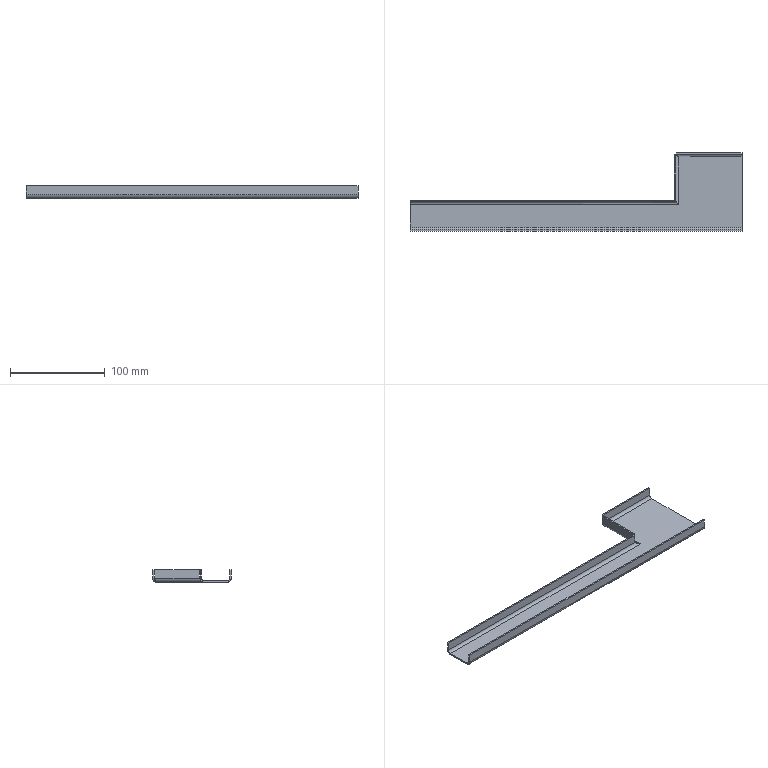Part | SolidWorks | features BaseBody 1 | 1 solid | 40 faces | box 350 x 83 x 13.5 mm | volume 34272 mm3 | plane 28 | cylinder 8 | spline 4 | commonest cylinder face diameters 6 x4 9 x4
STEP:
#1=CARTESIAN_POINT('',(105.707,41.5,12.));
#2=VERTEX_POINT('',#1);
#3=CARTESIAN_POINT('',(105.707,40.,12.));
#4=VERTEX_POINT('',#3);
#5=CARTESIAN_POINT('',(105.707,41.5,12.));
#6=DIRECTION('',(0.,-1.,0.));
#7=VECTOR('',#6,1000.);
#8=LINE('',#5,#7);
#9=EDGE_CURVE('',#2,#4,#8,.T.);
#10=ORIENTED_EDGE('',*,*,#9,.F.);
#11=CARTESIAN_POINT('',(105.707,41.5,3.));
#12=VERTEX_POINT('',#11);
#13=CARTESIAN_POINT('',(105.707,41.5,0.));
#14=DIRECTION('',(0.,0.,1.));
#15=VECTOR('',#14,1000.);
#16=LINE('',#13,#15);
#17=EDGE_CURVE('',#12,#2,#16,.T.);
#18=ORIENTED_EDGE('',*,*,#17,.F.);
#19=CARTESIAN_POINT('',(105.707,40.,3.));
#20=VERTEX_POINT('',#19);
#21=CARTESIAN_POINT('',(105.707,40.,3.));
#22=DIRECTION('',(0.,-1.,0.));
#23=VECTOR('',#22,1000.);
#24=LINE('',#21,#23);
#25=EDGE_CURVE('',#12,#20,#24,.T.);
#26=ORIENTED_EDGE('',*,*,#25,.T.);
#27=CARTESIAN_POINT('',(105.707,40.,0.));
#28=DIRECTION('',(0.,0.,1.));
#29=VECTOR('',#28,1000.);
#30=LINE('',#27,#29);
#31=EDGE_CURVE('',#20,#4,#30,.T.);
#32=ORIENTED_EDGE('',*,*,#31,.T.);
#33=EDGE_LOOP('',(#10,#18,#26,#32));
#34=FACE_OUTER_BOUND('',#33,.T.);
#35=CARTESIAN_POINT('',(105.707,40.,0.));
#36=DIRECTION('',(1.,0.,0.));
#37=DIRECTION('',(0.,1.,0.));
#38=AXIS2_PLACEMENT_3D('',#35,#36,#37);
#39=PLANE('',#38);
#40=ADVANCED_FACE('',(#34),#39,.F.);
#41=CARTESIAN_POINT('',(175.,41.5,12.));
#42=VERTEX_POINT('',#41);
#43=CARTESIAN_POINT('',(175.,41.5,12.));
#44=DIRECTION('',(1.,0.,0.));
#45=VECTOR('',#44,1000.);
#46=LINE('',#43,#45);
#47=EDGE_CURVE('',#2,#42,#46,.T.);
#48=ORIENTED_EDGE('',*,*,#47,.F.);
#49=ORIENTED_EDGE('',*,*,#9,.T.);
#50=CARTESIAN_POINT('',(175.,40.,12.));
#51=VERTEX_POINT('',#50);
#52=CARTESIAN_POINT('',(175.,40.,12.));
#53=DIRECTION('',(1.,0.,0.));
#54=VECTOR('',#53,1000.);
#55=LINE('',#52,#54);
#56=EDGE_CURVE('',#4,#51,#55,.T.);
#57=ORIENTED_EDGE('',*,*,#56,.T.);
#58=CARTESIAN_POINT('',(175.,41.5,12.));
#59=DIRECTION('',(0.,-1.,0.));
#60=VECTOR('',#59,1000.);
#61=LINE('',#58,#60);
#62=EDGE_CURVE('',#42,#51,#61,.T.);
#63=ORIENTED_EDGE('',*,*,#62,.F.);
#64=EDGE_LOOP('',(#48,#49,#57,#63));
#65=FACE_OUTER_BOUND('',#64,.T.);
#66=CARTESIAN_POINT('',(175.,41.5,12.));
#67=DIRECTION('',(0.,0.,-1.));
#68=DIRECTION('',(0.,-1.,0.));
#69=AXIS2_PLACEMENT_3D('',#66,#67,#68);
#70=PLANE('',#69);
#71=ADVANCED_FACE('',(#65),#70,.F.);
#72=ORIENTED_EDGE('',*,*,#31,.F.);
#73=CARTESIAN_POINT('',(175.,40.,3.));
#74=VERTEX_POINT('',#73);
#75=CARTESIAN_POINT('',(175.,40.,3.));
#76=DIRECTION('',(-1.,0.,0.));
#77=VECTOR('',#76,1000.);
#78=LINE('',#75,#77);
#79=EDGE_CURVE('',#74,#20,#78,.T.);
#80=ORIENTED_EDGE('',*,*,#79,.F.);
#81=CARTESIAN_POINT('',(175.,40.,0.));
#82=DIRECTION('',(0.,0.,-1.));
#83=VECTOR('',#82,1000.);
#84=LINE('',#81,#83);
#85=EDGE_CURVE('',#51,#74,#84,.T.);
#86=ORIENTED_EDGE('',*,*,#85,.F.);
#87=ORIENTED_EDGE('',*,*,#56,.F.);
#88=EDGE_LOOP('',(#72,#80,#86,#87));
#89=FACE_OUTER_BOUND('',#88,.T.);
#90=CARTESIAN_POINT('',(0.,40.,0.));
#91=DIRECTION('',(0.,-1.,0.));
#92=DIRECTION('',(-1.,0.,0.));
#93=AXIS2_PLACEMENT_3D('',#90,#91,#92);
#94=PLANE('',#93);
#95=ADVANCED_FACE('',(#89),#94,.T.);
#96=CARTESIAN_POINT('',(175.,41.5,3.));
#97=VERTEX_POINT('',#96);
#98=CARTESIAN_POINT('',(0.,41.5,3.));
#99=DIRECTION('',(1.,0.,0.));
#100=VECTOR('',#99,1000.);
#101=LINE('',#98,#100);
#102=EDGE_CURVE('',#12,#97,#101,.T.);
#103=ORIENTED_EDGE('',*,*,#102,.F.);
#104=ORIENTED_EDGE('',*,*,#17,.T.);
#105=ORIENTED_EDGE('',*,*,#47,.T.);
#106=CARTESIAN_POINT('',(175.,41.5,0.));
#107=DIRECTION('',(0.,0.,-1.));
#108=VECTOR('',#107,1000.);
#109=LINE('',#106,#108);
#110=EDGE_CURVE('',#42,#97,#109,.T.);
#111=ORIENTED_EDGE('',*,*,#110,.T.);
#112=EDGE_LOOP('',(#103,#104,#105,#111));
#113=FACE_OUTER_BOUND('',#112,.T.);
#114=CARTESIAN_POINT('',(0.,41.5,0.));
#115=DIRECTION('',(0.,-1.,0.));
#116=DIRECTION('',(-1.,0.,0.));
#117=AXIS2_PLACEMENT_3D('',#114,#115,#116);
#118=PLANE('',#117);
#119=ADVANCED_FACE('',(#113),#118,.F.);
#120=CARTESIAN_POINT('',(175.,40.,3.));
#121=DIRECTION('',(0.,1.,0.));
#122=VECTOR('',#121,1000.);
#123=LINE('',#120,#122);
#124=EDGE_CURVE('',#74,#97,#123,.T.);
#125=ORIENTED_EDGE('',*,*,#124,.T.);
#126=ORIENTED_EDGE('',*,*,#110,.F.);
#127=ORIENTED_EDGE('',*,*,#62,.T.);
#128=ORIENTED_EDGE('',*,*,#85,.T.);
#129=EDGE_LOOP('',(#125,#126,#127,#128));
#130=FACE_OUTER_BOUND('',#129,.T.);
#131=CARTESIAN_POINT('',(175.,41.5,0.));
#132=DIRECTION('',(-1.,0.,0.));
#133=DIRECTION('',(0.,0.,1.));
#134=AXIS2_PLACEMENT_3D('',#131,#132,#133);
#135=PLANE('',#134);
#136=ADVANCED_FACE('',(#130),#135,.F.);
#137=CARTESIAN_POINT('',(108.,37.,0.));
#138=VERTEX_POINT('',#137);
#139=CARTESIAN_POINT('',(175.,37.,0.));
#140=VERTEX_POINT('',#139);
#141=CARTESIAN_POINT('',(105.707,37.,0.));
#142=DIRECTION('',(1.,0.,0.));
#143=VECTOR('',#142,1000.);
#144=LINE('',#141,#143);
#145=EDGE_CURVE('',#138,#140,#144,.T.);
#146=ORIENTED_EDGE('',*,*,#145,.T.);
#147=CARTESIAN_POINT('',(175.,37.,3.));
#148=DIRECTION('',(1.,0.,0.));
#149=DIRECTION('',(0.,0.,1.));
#150=AXIS2_PLACEMENT_3D('',#147,#148,#149);
#151=CIRCLE('',#150,3.);
#152=EDGE_CURVE('',#140,#74,#151,.T.);
#153=ORIENTED_EDGE('',*,*,#152,.T.);
#154=ORIENTED_EDGE('',*,*,#79,.T.);
#155=CARTESIAN_POINT('',(105.707,40.,3.));
#156=CARTESIAN_POINT('',(105.898,40.,2.607));
#157=CARTESIAN_POINT('',(106.089,39.922,2.215));
#158=CARTESIAN_POINT('',(106.471,39.621,1.489));
#159=CARTESIAN_POINT('',(106.662,39.399,1.156));
#160=CARTESIAN_POINT('',(107.045,38.844,0.601));
#161=CARTESIAN_POINT('',(107.236,38.511,0.3786));
#162=CARTESIAN_POINT('',(107.618,37.785,0.07808));
#163=CARTESIAN_POINT('',(107.809,37.393,0.));
#164=CARTESIAN_POINT('',(108.,37.,0.));
#165=B_SPLINE_CURVE_WITH_KNOTS('',3,(#155,#156,#157,#158,#159,#160,#161,#162,#163,#164),.UNSPECIFIED.,.F.,.F.,(4,2,2,2,4),(0.,0.25,0.5,0.75,1.),.UNSPECIFIED.);
#166=EDGE_CURVE('',#20,#138,#165,.T.);
#167=ORIENTED_EDGE('',*,*,#166,.T.);
#168=EDGE_LOOP('',(#146,#153,#154,#167));
#169=FACE_OUTER_BOUND('',#168,.T.);
#170=CARTESIAN_POINT('',(105.707,37.,3.));
#171=DIRECTION('',(-1.,0.,0.));
#172=DIRECTION('',(0.,1.,0.));
#173=AXIS2_PLACEMENT_3D('',#170,#171,#172);
#174=CYLINDRICAL_SURFACE('',#173,3.);
#175=ADVANCED_FACE('',(#169),#174,.F.);
#176=CARTESIAN_POINT('',(108.,37.,-1.5));
#177=VERTEX_POINT('',#176);
#178=CARTESIAN_POINT('',(175.,37.,-1.5));
#179=VERTEX_POINT('',#178);
#180=CARTESIAN_POINT('',(105.707,37.,-1.5));
#181=DIRECTION('',(1.,0.,0.));
#182=VECTOR('',#181,1000.);
#183=LINE('',#180,#182);
#184=EDGE_CURVE('',#177,#179,#183,.T.);
#185=ORIENTED_EDGE('',*,*,#184,.F.);
#186=CARTESIAN_POINT('',(105.707,41.5,3.));
#187=CARTESIAN_POINT('',(105.898,41.5,2.411));
#188=CARTESIAN_POINT('',(106.089,41.383,1.822));
#189=CARTESIAN_POINT('',(106.471,40.932,0.7337));
#190=CARTESIAN_POINT('',(106.662,40.599,0.2345));
#191=CARTESIAN_POINT('',(107.045,39.765,-0.5985));
#192=CARTESIAN_POINT('',(107.236,39.266,-0.932));
#193=CARTESIAN_POINT('',(107.618,38.178,-1.383));
#194=CARTESIAN_POINT('',(107.809,37.589,-1.5));
#195=CARTESIAN_POINT('',(108.,37.,-1.5));
#196=B_SPLINE_CURVE_WITH_KNOTS('',3,(#186,#187,#188,#189,#190,#191,#192,#193,#194,#195),.UNSPECIFIED.,.F.,.F.,(4,2,2,2,4),(0.,0.25,0.5,0.75,1.),.UNSPECIFIED.);
#197=EDGE_CURVE('',#12,#177,#196,.T.);
#198=ORIENTED_EDGE('',*,*,#197,.F.);
#199=ORIENTED_EDGE('',*,*,#102,.T.);
#200=CARTESIAN_POINT('',(175.,37.,3.));
#201=DIRECTION('',(1.,0.,0.));
#202=DIRECTION('',(0.,0.,1.));
#203=AXIS2_PLACEMENT_3D('',#200,#201,#202);
#204=CIRCLE('',#203,4.5);
#205=EDGE_CURVE('',#179,#97,#204,.T.);
#206=ORIENTED_EDGE('',*,*,#205,.F.);
#207=EDGE_LOOP('',(#185,#198,#199,#206));
#208=FACE_OUTER_BOUND('',#207,.T.);
#209=CARTESIAN_POINT('',(105.707,37.,3.));
#210=DIRECTION('',(-1.,0.,0.));
#211=DIRECTION('',(0.,1.,0.));
#212=AXIS2_PLACEMENT_3D('',#209,#210,#211);
#213=CYLINDRICAL_SURFACE('',#212,4.5);
#214=ADVANCED_FACE('',(#208),#213,.T.);
#215=ORIENTED_EDGE('',*,*,#166,.F.);
#216=ORIENTED_EDGE('',*,*,#25,.F.);
#217=ORIENTED_EDGE('',*,*,#197,.T.);
#218=CARTESIAN_POINT('',(108.,37.,0.));
#219=DIRECTION('',(0.,0.,-1.));
#220=VECTOR('',#219,1000.);
#221=LINE('',#218,#220);
#222=EDGE_CURVE('',#138,#177,#221,.T.);
#223=ORIENTED_EDGE('',*,*,#222,.F.);
#224=EDGE_LOOP('',(#215,#216,#217,#223));
#225=FACE_OUTER_BOUND('',#224,.T.);
#226=CARTESIAN_POINT('',(105.707,41.515,3.));
#227=CARTESIAN_POINT('',(105.898,41.515,2.409));
#228=CARTESIAN_POINT('',(106.089,41.397,1.818));
#229=CARTESIAN_POINT('',(106.471,40.945,0.7262));
#230=CARTESIAN_POINT('',(106.662,40.61,0.2253));
#231=CARTESIAN_POINT('',(107.045,39.775,-0.6105));
#232=CARTESIAN_POINT('',(107.236,39.274,-0.9451));
#233=CARTESIAN_POINT('',(107.618,38.182,-1.397));
#234=CARTESIAN_POINT('',(107.809,37.591,-1.515));
#235=CARTESIAN_POINT('',(108.,37.,-1.515));
#236=CARTESIAN_POINT('',(105.707,41.5,3.));
#237=CARTESIAN_POINT('',(105.898,41.5,2.411));
#238=CARTESIAN_POINT('',(106.089,41.383,1.822));
#239=CARTESIAN_POINT('',(106.471,40.932,0.7337));
#240=CARTESIAN_POINT('',(106.662,40.599,0.2345));
#241=CARTESIAN_POINT('',(107.045,39.765,-0.5985));
#242=CARTESIAN_POINT('',(107.236,39.266,-0.932));
#243=CARTESIAN_POINT('',(107.618,38.178,-1.383));
#244=CARTESIAN_POINT('',(107.809,37.589,-1.5));
#245=CARTESIAN_POINT('',(108.,37.,-1.5));
#246=CARTESIAN_POINT('',(105.707,40.,3.));
#247=CARTESIAN_POINT('',(105.898,40.,2.607));
#248=CARTESIAN_POINT('',(106.089,39.922,2.215));
#249=CARTESIAN_POINT('',(106.471,39.621,1.489));
#250=CARTESIAN_POINT('',(106.662,39.399,1.156));
#251=CARTESIAN_POINT('',(107.045,38.844,0.601));
#252=CARTESIAN_POINT('',(107.236,38.511,0.3786));
#253=CARTESIAN_POINT('',(107.618,37.785,0.07808));
#254=CARTESIAN_POINT('',(107.809,37.393,0.));
#255=CARTESIAN_POINT('',(108.,37.,0.));
#256=CARTESIAN_POINT('',(105.707,39.985,3.));
#257=CARTESIAN_POINT('',(105.898,39.985,2.609));
#258=CARTESIAN_POINT('',(106.089,39.907,2.219));
#259=CARTESIAN_POINT('',(106.471,39.608,1.497));
#260=CARTESIAN_POINT('',(106.662,39.387,1.166));
#261=CARTESIAN_POINT('',(107.045,38.834,0.6131));
#262=CARTESIAN_POINT('',(107.236,38.503,0.3919));
#263=CARTESIAN_POINT('',(107.618,37.781,0.09284));
#264=CARTESIAN_POINT('',(107.809,37.391,0.01515));
#265=CARTESIAN_POINT('',(108.,37.,0.01515));
#266=B_SPLINE_SURFACE_WITH_KNOTS('',1,3,((#226,#227,#228,#229,#230,#231,#232,#233,#234,#235),(#236,#237,#238,#239,#240,#241,#242,#243,#244,#245),(#246,#247,#248,#249,#250,#251,#252,#253,#254,#255),(#256,#257,#258,#259,#260,#261,#262,#263,#264,#265)),.UNSPECIFIED.,.F.,.F.,.F.,(2,1,1,2),(4,2,2,2,4),(-0.01,0.,1.,1.01),(0.,0.25,0.5,0.75,1.),.UNSPECIFIED.);
#267=ADVANCED_FACE('',(#225),#266,.F.);
#268=ORIENTED_EDGE('',*,*,#124,.F.);
#269=ORIENTED_EDGE('',*,*,#152,.F.);
#270=CARTESIAN_POINT('',(175.,37.,0.));
#271=DIRECTION('',(0.,0.,-1.));
#272=VECTOR('',#271,1000.);
#273=LINE('',#270,#272);
#274=EDGE_CURVE('',#140,#179,#273,.T.);
#275=ORIENTED_EDGE('',*,*,#274,.T.);
#276=ORIENTED_EDGE('',*,*,#205,.T.);
#277=EDGE_LOOP('',(#268,#269,#275,#276));
#278=FACE_OUTER_BOUND('',#277,.T.);
#279=CARTESIAN_POINT('',(175.,37.,3.));
#280=DIRECTION('',(1.,0.,0.));
#281=DIRECTION('',(0.,1.,0.));
#282=AXIS2_PLACEMENT_3D('',#279,#280,#281);
#283=PLANE('',#282);
#284=ADVANCED_FACE('',(#278),#283,.T.);
#285=CARTESIAN_POINT('',(103.5,-7.793,12.));
#286=VERTEX_POINT('',#285);
#287=CARTESIAN_POINT('',(105.,-7.793,12.));
#288=VERTEX_POINT('',#287);
#289=CARTESIAN_POINT('',(103.5,-7.793,12.));
#290=DIRECTION('',(1.,0.,0.));
#291=VECTOR('',#290,1000.);
#292=LINE('',#289,#291);
#293=EDGE_CURVE('',#286,#288,#292,.T.);
#294=ORIENTED_EDGE('',*,*,#293,.F.);
#295=CARTESIAN_POINT('',(103.5,-7.793,3.));
#296=VERTEX_POINT('',#295);
#297=CARTESIAN_POINT('',(103.5,-7.793,0.));
#298=DIRECTION('',(0.,0.,1.));
#299=VECTOR('',#298,1000.);
#300=LINE('',#297,#299);
#301=EDGE_CURVE('',#296,#286,#300,.T.);
#302=ORIENTED_EDGE('',*,*,#301,.F.);
#303=CARTESIAN_POINT('',(105.,-7.793,3.));
#304=VERTEX_POINT('',#303);
#305=CARTESIAN_POINT('',(105.,-7.793,3.));
#306=DIRECTION('',(1.,0.,0.));
#307=VECTOR('',#306,1000.);
#308=LINE('',#305,#307);
#309=EDGE_CURVE('',#296,#304,#308,.T.);
#310=ORIENTED_EDGE('',*,*,#309,.T.);
#311=CARTESIAN_POINT('',(105.,-7.793,0.));
#312=DIRECTION('',(0.,0.,1.));
#313=VECTOR('',#312,1000.);
#314=LINE('',#311,#313);
#315=EDGE_CURVE('',#304,#288,#314,.T.);
#316=ORIENTED_EDGE('',*,*,#315,.T.);
#317=EDGE_LOOP('',(#294,#302,#310,#316));
#318=FACE_OUTER_BOUND('',#317,.T.);
#319=CARTESIAN_POINT('',(105.,-7.793,0.));
#320=DIRECTION('',(0.,1.,0.));
#321=DIRECTION('',(1.,0.,0.));
#322=AXIS2_PLACEMENT_3D('',#319,#320,#321);
#323=PLANE('',#322);
#324=ADVANCED_FACE('',(#318),#323,.F.);
#325=CARTESIAN_POINT('',(103.5,39.293,12.));
#326=VERTEX_POINT('',#325);
#327=CARTESIAN_POINT('',(103.5,40.,12.));
#328=DIRECTION('',(0.,1.,0.));
#329=VECTOR('',#328,1000.);
#330=LINE('',#327,#329);
#331=EDGE_CURVE('',#286,#326,#330,.T.);
#332=ORIENTED_EDGE('',*,*,#331,.F.);
#333=ORIENTED_EDGE('',*,*,#293,.T.);
#334=CARTESIAN_POINT('',(105.,39.293,12.));
#335=VERTEX_POINT('',#334);
#336=CARTESIAN_POINT('',(105.,40.,12.));
#337=DIRECTION('',(0.,1.,0.));
#338=VECTOR('',#337,1000.);
#339=LINE('',#336,#338);
#340=EDGE_CURVE('',#288,#335,#339,.T.);
#341=ORIENTED_EDGE('',*,*,#340,.T.);
#342=CARTESIAN_POINT('',(103.5,39.293,12.));
#343=DIRECTION('',(1.,0.,0.));
#344=VECTOR('',#343,1000.);
#345=LINE('',#342,#344);
#346=EDGE_CURVE('',#326,#335,#345,.T.);
#347=ORIENTED_EDGE('',*,*,#346,.F.);
#348=EDGE_LOOP('',(#332,#333,#341,#347));
#349=FACE_OUTER_BOUND('',#348,.T.);
#350=CARTESIAN_POINT('',(103.5,40.,12.));
#351=DIRECTION('',(0.,0.,-1.));
#352=DIRECTION('',(0.,-1.,0.));
#353=AXIS2_PLACEMENT_3D('',#350,#351,#352);
#354=PLANE('',#353);
#355=ADVANCED_FACE('',(#349),#354,.F.);
#356=ORIENTED_EDGE('',*,*,#315,.F.);
#357=CARTESIAN_POINT('',(105.,39.293,3.));
#358=VERTEX_POINT('',#357);
#359=CARTESIAN_POINT('',(105.,40.,3.));
#360=DIRECTION('',(0.,-1.,0.));
#361=VECTOR('',#360,1000.);
#362=LINE('',#359,#361);
#363=EDGE_CURVE('',#358,#304,#362,.T.);
#364=ORIENTED_EDGE('',*,*,#363,.F.);
#365=CARTESIAN_POINT('',(105.,39.293,0.));
#366=DIRECTION('',(0.,0.,1.));
#367=VECTOR('',#366,1000.);
#368=LINE('',#365,#367);
#369=EDGE_CURVE('',#358,#335,#368,.T.);
#370=ORIENTED_EDGE('',*,*,#369,.T.);
#371=ORIENTED_EDGE('',*,*,#340,.F.);
#372=EDGE_LOOP('',(#356,#364,#370,#371));
#373=FACE_OUTER_BOUND('',#372,.T.);
#374=CARTESIAN_POINT('',(105.,0.,0.));
#375=DIRECTION('',(1.,0.,0.));
#376=DIRECTION('',(0.,0.,1.));
#377=AXIS2_PLACEMENT_3D('',#374,#375,#376);
#378=PLANE('',#377);
#379=ADVANCED_FACE('',(#373),#378,.T.);
#380=CARTESIAN_POINT('',(103.5,39.293,3.));
#381=VERTEX_POINT('',#380);
#382=CARTESIAN_POINT('',(103.5,0.,3.));
#383=DIRECTION('',(0.,1.,0.));
#384=VECTOR('',#383,1000.);
#385=LINE('',#382,#384);
#386=EDGE_CURVE('',#296,#381,#385,.T.);
#387=ORIENTED_EDGE('',*,*,#386,.F.);
#388=ORIENTED_EDGE('',*,*,#301,.T.);
#389=ORIENTED_EDGE('',*,*,#331,.T.);
#390=CARTESIAN_POINT('',(103.5,39.293,0.));
#391=DIRECTION('',(0.,0.,1.));
#392=VECTOR('',#391,1000.);
#393=LINE('',#390,#392);
#394=EDGE_CURVE('',#381,#326,#393,.T.);
#395=ORIENTED_EDGE('',*,*,#394,.F.);
#396=EDGE_LOOP('',(#387,#388,#389,#395));
#397=FACE_OUTER_BOUND('',#396,.T.);
#398=CARTESIAN_POINT('',(103.5,0.,0.));
#399=DIRECTION('',(1.,0.,0.));
#400=DIRECTION('',(0.,0.,1.));
#401=AXIS2_PLACEMENT_3D('',#398,#399,#400);
#402=PLANE('',#401);
#403=ADVANCED_FACE('',(#397),#402,.F.);
#404=ORIENTED_EDGE('',*,*,#394,.T.);
#405=ORIENTED_EDGE('',*,*,#346,.T.);
#406=ORIENTED_EDGE('',*,*,#369,.F.);
#407=CARTESIAN_POINT('',(105.,39.293,3.));
#408=DIRECTION('',(1.,0.,0.));
#409=VECTOR('',#408,1000.);
#410=LINE('',#407,#409);
#411=EDGE_CURVE('',#381,#358,#410,.T.);
#412=ORIENTED_EDGE('',*,*,#411,.F.);
#413=EDGE_LOOP('',(#404,#405,#406,#412));
#414=FACE_OUTER_BOUND('',#413,.T.);
#415=CARTESIAN_POINT('',(105.,39.293,0.));
#416=DIRECTION('',(0.,1.,0.));
#417=DIRECTION('',(1.,0.,0.));
#418=AXIS2_PLACEMENT_3D('',#415,#416,#417);
#419=PLANE('',#418);
#420=ADVANCED_FACE('',(#414),#419,.T.);
#421=CARTESIAN_POINT('',(108.,-13.,0.));
#422=VERTEX_POINT('',#421);
#423=CARTESIAN_POINT('',(108.,-13.,0.));
#424=DIRECTION('',(0.,1.,0.));
#425=VECTOR('',#424,1000.);
#426=LINE('',#423,#425);
#427=EDGE_CURVE('',#422,#138,#426,.T.);
#428=ORIENTED_EDGE('',*,*,#427,.T.);
#429=CARTESIAN_POINT('',(108.,37.,0.));
#430=CARTESIAN_POINT('',(107.607,37.191,0.));
#431=CARTESIAN_POINT('',(107.215,37.382,0.07808));
#432=CARTESIAN_POINT('',(106.489,37.764,0.3786));
#433=CARTESIAN_POINT('',(106.156,37.955,0.601));
#434=CARTESIAN_POINT('',(105.601,38.338,1.156));
#435=CARTESIAN_POINT('',(105.379,38.529,1.489));
#436=CARTESIAN_POINT('',(105.078,38.911,2.215));
#437=CARTESIAN_POINT('',(105.,39.102,2.607));
#438=CARTESIAN_POINT('',(105.,39.293,3.));
#439=B_SPLINE_CURVE_WITH_KNOTS('',3,(#429,#430,#431,#432,#433,#434,#435,#436,#437,#438),.UNSPECIFIED.,.F.,.F.,(4,2,2,2,4),(0.,0.25,0.5,0.75,1.),.UNSPECIFIED.);
#440=EDGE_CURVE('',#138,#358,#439,.T.);
#441=ORIENTED_EDGE('',*,*,#440,.T.);
#442=ORIENTED_EDGE('',*,*,#363,.T.);
#443=CARTESIAN_POINT('',(105.,-7.793,3.));
#444=CARTESIAN_POINT('',(105.,-8.227,2.607));
#445=CARTESIAN_POINT('',(105.078,-8.661,2.215));
#446=CARTESIAN_POINT('',(105.379,-9.529,1.489));
#447=CARTESIAN_POINT('',(105.601,-9.963,1.156));
#448=CARTESIAN_POINT('',(106.156,-10.83,0.601));
#449=CARTESIAN_POINT('',(106.489,-11.264,0.3786));
#450=CARTESIAN_POINT('',(107.215,-12.132,0.07808));
#451=CARTESIAN_POINT('',(107.607,-12.566,0.));
#452=CARTESIAN_POINT('',(108.,-13.,0.));
#453=B_SPLINE_CURVE_WITH_KNOTS('',3,(#443,#444,#445,#446,#447,#448,#449,#450,#451,#452),.UNSPECIFIED.,.F.,.F.,(4,2,2,2,4),(0.,0.25,0.5,0.75,1.),.UNSPECIFIED.);
#454=EDGE_CURVE('',#304,#422,#453,.T.);
#455=ORIENTED_EDGE('',*,*,#454,.T.);
#456=EDGE_LOOP('',(#428,#441,#442,#455));
#457=FACE_OUTER_BOUND('',#456,.T.);
#458=CARTESIAN_POINT('',(108.,-13.,3.));
#459=DIRECTION('',(0.,-1.,0.));
#460=DIRECTION('',(-1.,0.,0.));
#461=AXIS2_PLACEMENT_3D('',#458,#459,#460);
#462=CYLINDRICAL_SURFACE('',#461,3.);
#463=ADVANCED_FACE('',(#457),#462,.F.);
#464=CARTESIAN_POINT('',(108.,-13.,-1.5));
#465=VERTEX_POINT('',#464);
#466=CARTESIAN_POINT('',(108.,-13.,-1.5));
#467=DIRECTION('',(0.,1.,0.));
#468=VECTOR('',#467,1000.);
#469=LINE('',#466,#468);
#470=EDGE_CURVE('',#465,#177,#469,.T.);
#471=ORIENTED_EDGE('',*,*,#470,.F.);
#472=CARTESIAN_POINT('',(103.5,-7.793,3.));
#473=CARTESIAN_POINT('',(103.5,-8.227,2.411));
#474=CARTESIAN_POINT('',(103.617,-8.661,1.822));
#475=CARTESIAN_POINT('',(104.068,-9.529,0.7337));
#476=CARTESIAN_POINT('',(104.401,-9.963,0.2345));
#477=CARTESIAN_POINT('',(105.235,-10.83,-0.5985));
#478=CARTESIAN_POINT('',(105.734,-11.264,-0.932));
#479=CARTESIAN_POINT('',(106.822,-12.132,-1.383));
#480=CARTESIAN_POINT('',(107.411,-12.566,-1.5));
#481=CARTESIAN_POINT('',(108.,-13.,-1.5));
#482=B_SPLINE_CURVE_WITH_KNOTS('',3,(#472,#473,#474,#475,#476,#477,#478,#479,#480,#481),.UNSPECIFIED.,.F.,.F.,(4,2,2,2,4),(0.,0.25,0.5,0.75,1.),.UNSPECIFIED.);
#483=EDGE_CURVE('',#296,#465,#482,.T.);
#484=ORIENTED_EDGE('',*,*,#483,.F.);
#485=ORIENTED_EDGE('',*,*,#386,.T.);
#486=CARTESIAN_POINT('',(108.,37.,-1.5));
#487=CARTESIAN_POINT('',(107.411,37.191,-1.5));
#488=CARTESIAN_POINT('',(106.822,37.382,-1.383));
#489=CARTESIAN_POINT('',(105.734,37.764,-0.932));
#490=CARTESIAN_POINT('',(105.235,37.955,-0.5985));
#491=CARTESIAN_POINT('',(104.401,38.338,0.2345));
#492=CARTESIAN_POINT('',(104.068,38.529,0.7337));
#493=CARTESIAN_POINT('',(103.617,38.911,1.822));
#494=CARTESIAN_POINT('',(103.5,39.102,2.411));
#495=CARTESIAN_POINT('',(103.5,39.293,3.));
#496=B_SPLINE_CURVE_WITH_KNOTS('',3,(#486,#487,#488,#489,#490,#491,#492,#493,#494,#495),.UNSPECIFIED.,.F.,.F.,(4,2,2,2,4),(0.,0.25,0.5,0.75,1.),.UNSPECIFIED.);
#497=EDGE_CURVE('',#177,#381,#496,.T.);
#498=ORIENTED_EDGE('',*,*,#497,.F.);
#499=EDGE_LOOP('',(#471,#484,#485,#498));
#500=FACE_OUTER_BOUND('',#499,.T.);
#501=CARTESIAN_POINT('',(108.,-13.,3.));
#502=DIRECTION('',(0.,-1.,0.));
#503=DIRECTION('',(-1.,0.,0.));
#504=AXIS2_PLACEMENT_3D('',#501,#502,#503);
#505=CYLINDRICAL_SURFACE('',#504,4.5);
#506=ADVANCED_FACE('',(#500),#505,.T.);
#507=ORIENTED_EDGE('',*,*,#454,.F.);
#508=ORIENTED_EDGE('',*,*,#309,.F.);
#509=ORIENTED_EDGE('',*,*,#483,.T.);
#510=CARTESIAN_POINT('',(108.,-13.,0.));
#511=DIRECTION('',(0.,0.,-1.));
#512=VECTOR('',#511,1000.);
#513=LINE('',#510,#512);
#514=EDGE_CURVE('',#422,#465,#513,.T.);
#515=ORIENTED_EDGE('',*,*,#514,.F.);
#516=EDGE_LOOP('',(#507,#508,#509,#515));
#517=FACE_OUTER_BOUND('',#516,.T.);
#518=CARTESIAN_POINT('',(103.485,-7.793,3.));
#519=CARTESIAN_POINT('',(103.485,-8.227,2.409));
#520=CARTESIAN_POINT('',(103.603,-8.661,1.818));
#521=CARTESIAN_POINT('',(104.055,-9.529,0.7262));
#522=CARTESIAN_POINT('',(104.39,-9.963,0.2253));
#523=CARTESIAN_POINT('',(105.225,-10.83,-0.6105));
#524=CARTESIAN_POINT('',(105.726,-11.264,-0.9451));
#525=CARTESIAN_POINT('',(106.818,-12.132,-1.397));
#526=CARTESIAN_POINT('',(107.409,-12.566,-1.515));
#527=CARTESIAN_POINT('',(108.,-13.,-1.515));
#528=CARTESIAN_POINT('',(103.5,-7.793,3.));
#529=CARTESIAN_POINT('',(103.5,-8.227,2.411));
#530=CARTESIAN_POINT('',(103.617,-8.661,1.822));
#531=CARTESIAN_POINT('',(104.068,-9.529,0.7337));
#532=CARTESIAN_POINT('',(104.401,-9.963,0.2345));
#533=CARTESIAN_POINT('',(105.235,-10.83,-0.5985));
#534=CARTESIAN_POINT('',(105.734,-11.264,-0.932));
#535=CARTESIAN_POINT('',(106.822,-12.132,-1.383));
#536=CARTESIAN_POINT('',(107.411,-12.566,-1.5));
#537=CARTESIAN_POINT('',(108.,-13.,-1.5));
#538=CARTESIAN_POINT('',(105.,-7.793,3.));
#539=CARTESIAN_POINT('',(105.,-8.227,2.607));
#540=CARTESIAN_POINT('',(105.078,-8.661,2.215));
#541=CARTESIAN_POINT('',(105.379,-9.529,1.489));
#542=CARTESIAN_POINT('',(105.601,-9.963,1.156));
#543=CARTESIAN_POINT('',(106.156,-10.83,0.601));
#544=CARTESIAN_POINT('',(106.489,-11.264,0.3786));
#545=CARTESIAN_POINT('',(107.215,-12.132,0.07808));
#546=CARTESIAN_POINT('',(107.607,-12.566,0.));
#547=CARTESIAN_POINT('',(108.,-13.,0.));
#548=CARTESIAN_POINT('',(105.015,-7.793,3.));
#549=CARTESIAN_POINT('',(105.015,-8.227,2.609));
#550=CARTESIAN_POINT('',(105.093,-8.661,2.219));
#551=CARTESIAN_POINT('',(105.392,-9.529,1.497));
#552=CARTESIAN_POINT('',(105.613,-9.963,1.166));
#553=CARTESIAN_POINT('',(106.166,-10.83,0.6131));
#554=CARTESIAN_POINT('',(106.497,-11.264,0.3919));
#555=CARTESIAN_POINT('',(107.219,-12.132,0.09284));
#556=CARTESIAN_POINT('',(107.609,-12.566,0.01515));
#557=CARTESIAN_POINT('',(108.,-13.,0.01515));
#558=B_SPLINE_SURFACE_WITH_KNOTS('',1,3,((#518,#519,#520,#521,#522,#523,#524,#525,#526,#527),(#528,#529,#530,#531,#532,#533,#534,#535,#536,#537),(#538,#539,#540,#541,#542,#543,#544,#545,#546,#547),(#548,#549,#550,#551,#552,#553,#554,#555,#556,#557)),.UNSPECIFIED.,.F.,.F.,.F.,(2,1,1,2),(4,2,2,2,4),(-0.01,0.,1.,1.01),(0.,0.25,0.5,0.75,1.),.UNSPECIFIED.);
#559=ADVANCED_FACE('',(#517),#558,.F.);
#560=ORIENTED_EDGE('',*,*,#411,.T.);
#561=ORIENTED_EDGE('',*,*,#440,.F.);
#562=ORIENTED_EDGE('',*,*,#222,.T.);
#563=ORIENTED_EDGE('',*,*,#497,.T.);
#564=EDGE_LOOP('',(#560,#561,#562,#563));
#565=FACE_OUTER_BOUND('',#564,.T.);
#566=CARTESIAN_POINT('',(108.,37.,-1.515));
#567=CARTESIAN_POINT('',(107.409,37.191,-1.515));
#568=CARTESIAN_POINT('',(106.818,37.382,-1.397));
#569=CARTESIAN_POINT('',(105.726,37.764,-0.9451));
#570=CARTESIAN_POINT('',(105.225,37.955,-0.6105));
#571=CARTESIAN_POINT('',(104.39,38.338,0.2253));
#572=CARTESIAN_POINT('',(104.055,38.529,0.7262));
#573=CARTESIAN_POINT('',(103.603,38.911,1.818));
#574=CARTESIAN_POINT('',(103.485,39.102,2.409));
#575=CARTESIAN_POINT('',(103.485,39.293,3.));
#576=CARTESIAN_POINT('',(108.,37.,-1.5));
#577=CARTESIAN_POINT('',(107.411,37.191,-1.5));
#578=CARTESIAN_POINT('',(106.822,37.382,-1.383));
#579=CARTESIAN_POINT('',(105.734,37.764,-0.932));
#580=CARTESIAN_POINT('',(105.235,37.955,-0.5985));
#581=CARTESIAN_POINT('',(104.401,38.338,0.2345));
#582=CARTESIAN_POINT('',(104.068,38.529,0.7337));
#583=CARTESIAN_POINT('',(103.617,38.911,1.822));
#584=CARTESIAN_POINT('',(103.5,39.102,2.411));
#585=CARTESIAN_POINT('',(103.5,39.293,3.));
#586=CARTESIAN_POINT('',(108.,37.,0.));
#587=CARTESIAN_POINT('',(107.607,37.191,0.));
#588=CARTESIAN_POINT('',(107.215,37.382,0.07808));
#589=CARTESIAN_POINT('',(106.489,37.764,0.3786));
#590=CARTESIAN_POINT('',(106.156,37.955,0.601));
#591=CARTESIAN_POINT('',(105.601,38.338,1.156));
#592=CARTESIAN_POINT('',(105.379,38.529,1.489));
#593=CARTESIAN_POINT('',(105.078,38.911,2.215));
#594=CARTESIAN_POINT('',(105.,39.102,2.607));
#595=CARTESIAN_POINT('',(105.,39.293,3.));
#596=CARTESIAN_POINT('',(108.,37.,0.01515));
#597=CARTESIAN_POINT('',(107.609,37.191,0.01515));
#598=CARTESIAN_POINT('',(107.219,37.382,0.09284));
#599=CARTESIAN_POINT('',(106.497,37.764,0.3919));
#600=CARTESIAN_POINT('',(106.166,37.955,0.6131));
#601=CARTESIAN_POINT('',(105.613,38.338,1.166));
#602=CARTESIAN_POINT('',(105.392,38.529,1.497));
#603=CARTESIAN_POINT('',(105.093,38.911,2.219));
#604=CARTESIAN_POINT('',(105.015,39.102,2.609));
#605=CARTESIAN_POINT('',(105.015,39.293,3.));
#606=B_SPLINE_SURFACE_WITH_KNOTS('',1,3,((#566,#567,#568,#569,#570,#571,#572,#573,#574,#575),(#576,#577,#578,#579,#580,#581,#582,#583,#584,#585),(#586,#587,#588,#589,#590,#591,#592,#593,#594,#595),(#596,#597,#598,#599,#600,#601,#602,#603,#604,#605)),.UNSPECIFIED.,.F.,.F.,.F.,(2,1,1,2),(4,2,2,2,4),(-0.01,0.,1.,1.01),(0.,0.25,0.5,0.75,1.),.UNSPECIFIED.);
#607=ADVANCED_FACE('',(#565),#606,.F.);
#608=CARTESIAN_POINT('',(-175.,-10.,3.));
#609=VERTEX_POINT('',#608);
#610=CARTESIAN_POINT('',(-175.,-8.5,3.));
#611=VERTEX_POINT('',#610);
#612=CARTESIAN_POINT('',(-175.,-10.,3.));
#613=DIRECTION('',(0.,1.,0.));
#614=VECTOR('',#613,1000.);
#615=LINE('',#612,#614);
#616=EDGE_CURVE('',#609,#611,#615,.T.);
#617=ORIENTED_EDGE('',*,*,#616,.F.);
#618=CARTESIAN_POINT('',(-175.,-10.,12.));
#619=VERTEX_POINT('',#618);
#620=CARTESIAN_POINT('',(-175.,-10.,12.));
#621=DIRECTION('',(0.,0.,1.));
#622=VECTOR('',#621,1000.);
#623=LINE('',#620,#622);
#624=EDGE_CURVE('',#609,#619,#623,.T.);
#625=ORIENTED_EDGE('',*,*,#624,.T.);
#626=CARTESIAN_POINT('',(-175.,-8.5,12.));
#627=VERTEX_POINT('',#626);
#628=CARTESIAN_POINT('',(-175.,-8.5,12.));
#629=DIRECTION('',(0.,-1.,0.));
#630=VECTOR('',#629,1000.);
#631=LINE('',#628,#630);
#632=EDGE_CURVE('',#627,#619,#631,.T.);
#633=ORIENTED_EDGE('',*,*,#632,.F.);
#634=CARTESIAN_POINT('',(-175.,-8.5,12.));
#635=DIRECTION('',(0.,0.,1.));
#636=VECTOR('',#635,1000.);
#637=LINE('',#634,#636);
#638=EDGE_CURVE('',#611,#627,#637,.T.);
#639=ORIENTED_EDGE('',*,*,#638,.F.);
#640=EDGE_LOOP('',(#617,#625,#633,#639));
#641=FACE_OUTER_BOUND('',#640,.T.);
#642=CARTESIAN_POINT('',(-175.,-8.5,12.));
#643=DIRECTION('',(1.,0.,0.));
#644=DIRECTION('',(0.,1.,0.));
#645=AXIS2_PLACEMENT_3D('',#642,#643,#644);
#646=PLANE('',#645);
#647=ADVANCED_FACE('',(#641),#646,.F.);
#648=CARTESIAN_POINT('',(102.793,-8.5,12.));
#649=VERTEX_POINT('',#648);
#650=CARTESIAN_POINT('',(102.793,-10.,12.));
#651=VERTEX_POINT('',#650);
#652=CARTESIAN_POINT('',(102.793,-8.5,12.));
#653=DIRECTION('',(0.,-1.,0.));
#654=VECTOR('',#653,1000.);
#655=LINE('',#652,#654);
#656=EDGE_CURVE('',#649,#651,#655,.T.);
#657=ORIENTED_EDGE('',*,*,#656,.F.);
#658=CARTESIAN_POINT('',(105.,-8.5,12.));
#659=DIRECTION('',(1.,0.,0.));
#660=VECTOR('',#659,1000.);
#661=LINE('',#658,#660);
#662=EDGE_CURVE('',#627,#649,#661,.T.);
#663=ORIENTED_EDGE('',*,*,#662,.F.);
#664=ORIENTED_EDGE('',*,*,#632,.T.);
#665=CARTESIAN_POINT('',(105.,-10.,12.));
#666=DIRECTION('',(1.,0.,0.));
#667=VECTOR('',#666,1000.);
#668=LINE('',#665,#667);
#669=EDGE_CURVE('',#619,#651,#668,.T.);
#670=ORIENTED_EDGE('',*,*,#669,.T.);
#671=EDGE_LOOP('',(#657,#663,#664,#670));
#672=FACE_OUTER_BOUND('',#671,.T.);
#673=CARTESIAN_POINT('',(105.,-8.5,12.));
#674=DIRECTION('',(0.,0.,-1.));
#675=DIRECTION('',(0.,-1.,0.));
#676=AXIS2_PLACEMENT_3D('',#673,#674,#675);
#677=PLANE('',#676);
#678=ADVANCED_FACE('',(#672),#677,.F.);
#679=CARTESIAN_POINT('',(102.793,-10.,3.));
#680=VERTEX_POINT('',#679);
#681=CARTESIAN_POINT('',(105.,-10.,3.));
#682=DIRECTION('',(-1.,0.,0.));
#683=VECTOR('',#682,1000.);
#684=LINE('',#681,#683);
#685=EDGE_CURVE('',#680,#609,#684,.T.);
#686=ORIENTED_EDGE('',*,*,#685,.F.);
#687=CARTESIAN_POINT('',(102.793,-10.,0.));
#688=DIRECTION('',(0.,0.,1.));
#689=VECTOR('',#688,1000.);
#690=LINE('',#687,#689);
#691=EDGE_CURVE('',#680,#651,#690,.T.);
#692=ORIENTED_EDGE('',*,*,#691,.T.);
#693=ORIENTED_EDGE('',*,*,#669,.F.);
#694=ORIENTED_EDGE('',*,*,#624,.F.);
#695=EDGE_LOOP('',(#686,#692,#693,#694));
#696=FACE_OUTER_BOUND('',#695,.T.);
#697=CARTESIAN_POINT('',(0.,-10.,0.));
#698=DIRECTION('',(0.,-1.,0.));
#699=DIRECTION('',(-1.,0.,0.));
#700=AXIS2_PLACEMENT_3D('',#697,#698,#699);
#701=PLANE('',#700);
#702=ADVANCED_FACE('',(#696),#701,.T.);
#703=CARTESIAN_POINT('',(102.793,-8.5,3.));
#704=VERTEX_POINT('',#703);
#705=CARTESIAN_POINT('',(102.793,-8.5,0.));
#706=DIRECTION('',(0.,0.,1.));
#707=VECTOR('',#706,1000.);
#708=LINE('',#705,#707);
#709=EDGE_CURVE('',#704,#649,#708,.T.);
#710=ORIENTED_EDGE('',*,*,#709,.F.);
#711=CARTESIAN_POINT('',(0.,-8.5,3.));
#712=DIRECTION('',(1.,0.,0.));
#713=VECTOR('',#712,1000.);
#714=LINE('',#711,#713);
#715=EDGE_CURVE('',#611,#704,#714,.T.);
#716=ORIENTED_EDGE('',*,*,#715,.F.);
#717=ORIENTED_EDGE('',*,*,#638,.T.);
#718=ORIENTED_EDGE('',*,*,#662,.T.);
#719=EDGE_LOOP('',(#710,#716,#717,#718));
#720=FACE_OUTER_BOUND('',#719,.T.);
#721=CARTESIAN_POINT('',(0.,-8.5,0.));
#722=DIRECTION('',(0.,-1.,0.));
#723=DIRECTION('',(-1.,0.,0.));
#724=AXIS2_PLACEMENT_3D('',#721,#722,#723);
#725=PLANE('',#724);
#726=ADVANCED_FACE('',(#720),#725,.F.);
#727=ORIENTED_EDGE('',*,*,#709,.T.);
#728=ORIENTED_EDGE('',*,*,#656,.T.);
#729=ORIENTED_EDGE('',*,*,#691,.F.);
#730=CARTESIAN_POINT('',(102.793,-10.,3.));
#731=DIRECTION('',(0.,-1.,0.));
#732=VECTOR('',#731,1000.);
#733=LINE('',#730,#732);
#734=EDGE_CURVE('',#704,#680,#733,.T.);
#735=ORIENTED_EDGE('',*,*,#734,.F.);
#736=EDGE_LOOP('',(#727,#728,#729,#735));
#737=FACE_OUTER_BOUND('',#736,.T.);
#738=CARTESIAN_POINT('',(102.793,-10.,0.));
#739=DIRECTION('',(1.,0.,0.));
#740=DIRECTION('',(0.,1.,0.));
#741=AXIS2_PLACEMENT_3D('',#738,#739,#740);
#742=PLANE('',#741);
#743=ADVANCED_FACE('',(#737),#742,.T.);
#744=CARTESIAN_POINT('',(-175.,-13.,0.));
#745=VERTEX_POINT('',#744);
#746=CARTESIAN_POINT('',(-175.,-13.,0.));
#747=DIRECTION('',(1.,0.,0.));
#748=VECTOR('',#747,1000.);
#749=LINE('',#746,#748);
#750=EDGE_CURVE('',#745,#422,#749,.T.);
#751=ORIENTED_EDGE('',*,*,#750,.T.);
#752=CARTESIAN_POINT('',(108.,-13.,0.));
#753=CARTESIAN_POINT('',(107.566,-12.607,0.));
#754=CARTESIAN_POINT('',(107.132,-12.215,0.07808));
#755=CARTESIAN_POINT('',(106.264,-11.489,0.3786));
#756=CARTESIAN_POINT('',(105.83,-11.156,0.601));
#757=CARTESIAN_POINT('',(104.963,-10.601,1.156));
#758=CARTESIAN_POINT('',(104.529,-10.379,1.489));
#759=CARTESIAN_POINT('',(103.661,-10.078,2.215));
#760=CARTESIAN_POINT('',(103.227,-10.,2.607));
#761=CARTESIAN_POINT('',(102.793,-10.,3.));
#762=B_SPLINE_CURVE_WITH_KNOTS('',3,(#752,#753,#754,#755,#756,#757,#758,#759,#760,#761),.UNSPECIFIED.,.F.,.F.,(4,2,2,2,4),(0.,0.25,0.5,0.75,1.),.UNSPECIFIED.);
#763=EDGE_CURVE('',#422,#680,#762,.T.);
#764=ORIENTED_EDGE('',*,*,#763,.T.);
#765=ORIENTED_EDGE('',*,*,#685,.T.);
#766=CARTESIAN_POINT('',(-175.,-13.,3.));
#767=DIRECTION('',(-1.,0.,0.));
#768=DIRECTION('',(0.,0.,1.));
#769=AXIS2_PLACEMENT_3D('',#766,#767,#768);
#770=CIRCLE('',#769,3.);
#771=EDGE_CURVE('',#609,#745,#770,.T.);
#772=ORIENTED_EDGE('',*,*,#771,.T.);
#773=EDGE_LOOP('',(#751,#764,#765,#772));
#774=FACE_OUTER_BOUND('',#773,.T.);
#775=CARTESIAN_POINT('',(-175.,-13.,3.));
#776=DIRECTION('',(-1.,0.,0.));
#777=DIRECTION('',(0.,1.,0.));
#778=AXIS2_PLACEMENT_3D('',#775,#776,#777);
#779=CYLINDRICAL_SURFACE('',#778,3.);
#780=ADVANCED_FACE('',(#774),#779,.F.);
#781=CARTESIAN_POINT('',(-175.,-13.,-1.5));
#782=VERTEX_POINT('',#781);
#783=CARTESIAN_POINT('',(-175.,-13.,-1.5));
#784=DIRECTION('',(1.,0.,0.));
#785=VECTOR('',#784,1000.);
#786=LINE('',#783,#785);
#787=EDGE_CURVE('',#782,#465,#786,.T.);
#788=ORIENTED_EDGE('',*,*,#787,.F.);
#789=CARTESIAN_POINT('',(-175.,-13.,3.));
#790=DIRECTION('',(-1.,0.,0.));
#791=DIRECTION('',(0.,0.,1.));
#792=AXIS2_PLACEMENT_3D('',#789,#790,#791);
#793=CIRCLE('',#792,4.5);
#794=EDGE_CURVE('',#611,#782,#793,.T.);
#795=ORIENTED_EDGE('',*,*,#794,.F.);
#796=ORIENTED_EDGE('',*,*,#715,.T.);
#797=CARTESIAN_POINT('',(108.,-13.,-1.5));
#798=CARTESIAN_POINT('',(107.566,-12.411,-1.5));
#799=CARTESIAN_POINT('',(107.132,-11.822,-1.383));
#800=CARTESIAN_POINT('',(106.264,-10.734,-0.932));
#801=CARTESIAN_POINT('',(105.83,-10.235,-0.5985));
#802=CARTESIAN_POINT('',(104.963,-9.401,0.2345));
#803=CARTESIAN_POINT('',(104.529,-9.068,0.7337));
#804=CARTESIAN_POINT('',(103.661,-8.617,1.822));
#805=CARTESIAN_POINT('',(103.227,-8.5,2.411));
#806=CARTESIAN_POINT('',(102.793,-8.5,3.));
#807=B_SPLINE_CURVE_WITH_KNOTS('',3,(#797,#798,#799,#800,#801,#802,#803,#804,#805,#806),.UNSPECIFIED.,.F.,.F.,(4,2,2,2,4),(0.,0.25,0.5,0.75,1.),.UNSPECIFIED.);
#808=EDGE_CURVE('',#465,#704,#807,.T.);
#809=ORIENTED_EDGE('',*,*,#808,.F.);
#810=EDGE_LOOP('',(#788,#795,#796,#809));
#811=FACE_OUTER_BOUND('',#810,.T.);
#812=CARTESIAN_POINT('',(-175.,-13.,3.));
#813=DIRECTION('',(-1.,0.,0.));
#814=DIRECTION('',(0.,1.,0.));
#815=AXIS2_PLACEMENT_3D('',#812,#813,#814);
#816=CYLINDRICAL_SURFACE('',#815,4.5);
#817=ADVANCED_FACE('',(#811),#816,.T.);
#818=ORIENTED_EDGE('',*,*,#771,.F.);
#819=ORIENTED_EDGE('',*,*,#616,.T.);
#820=ORIENTED_EDGE('',*,*,#794,.T.);
#821=CARTESIAN_POINT('',(-175.,-13.,0.));
#822=DIRECTION('',(0.,0.,-1.));
#823=VECTOR('',#822,1000.);
#824=LINE('',#821,#823);
#825=EDGE_CURVE('',#745,#782,#824,.T.);
#826=ORIENTED_EDGE('',*,*,#825,.F.);
#827=EDGE_LOOP('',(#818,#819,#820,#826));
#828=FACE_OUTER_BOUND('',#827,.T.);
#829=CARTESIAN_POINT('',(-175.,-13.,3.));
#830=DIRECTION('',(1.,0.,0.));
#831=DIRECTION('',(0.,1.,0.));
#832=AXIS2_PLACEMENT_3D('',#829,#830,#831);
#833=PLANE('',#832);
#834=ADVANCED_FACE('',(#828),#833,.F.);
#835=ORIENTED_EDGE('',*,*,#734,.T.);
#836=ORIENTED_EDGE('',*,*,#763,.F.);
#837=ORIENTED_EDGE('',*,*,#514,.T.);
#838=ORIENTED_EDGE('',*,*,#808,.T.);
#839=EDGE_LOOP('',(#835,#836,#837,#838));
#840=FACE_OUTER_BOUND('',#839,.T.);
#841=CARTESIAN_POINT('',(108.,-13.,-1.515));
#842=CARTESIAN_POINT('',(107.566,-12.409,-1.515));
#843=CARTESIAN_POINT('',(107.132,-11.818,-1.397));
#844=CARTESIAN_POINT('',(106.264,-10.726,-0.9451));
#845=CARTESIAN_POINT('',(105.83,-10.225,-0.6105));
#846=CARTESIAN_POINT('',(104.963,-9.39,0.2253));
#847=CARTESIAN_POINT('',(104.529,-9.055,0.7262));
#848=CARTESIAN_POINT('',(103.661,-8.603,1.818));
#849=CARTESIAN_POINT('',(103.227,-8.485,2.409));
#850=CARTESIAN_POINT('',(102.793,-8.485,3.));
#851=CARTESIAN_POINT('',(108.,-13.,-1.5));
#852=CARTESIAN_POINT('',(107.566,-12.411,-1.5));
#853=CARTESIAN_POINT('',(107.132,-11.822,-1.383));
#854=CARTESIAN_POINT('',(106.264,-10.734,-0.932));
#855=CARTESIAN_POINT('',(105.83,-10.235,-0.5985));
#856=CARTESIAN_POINT('',(104.963,-9.401,0.2345));
#857=CARTESIAN_POINT('',(104.529,-9.068,0.7337));
#858=CARTESIAN_POINT('',(103.661,-8.617,1.822));
#859=CARTESIAN_POINT('',(103.227,-8.5,2.411));
#860=CARTESIAN_POINT('',(102.793,-8.5,3.));
#861=CARTESIAN_POINT('',(108.,-13.,0.));
#862=CARTESIAN_POINT('',(107.566,-12.607,0.));
#863=CARTESIAN_POINT('',(107.132,-12.215,0.07808));
#864=CARTESIAN_POINT('',(106.264,-11.489,0.3786));
#865=CARTESIAN_POINT('',(105.83,-11.156,0.601));
#866=CARTESIAN_POINT('',(104.963,-10.601,1.156));
#867=CARTESIAN_POINT('',(104.529,-10.379,1.489));
#868=CARTESIAN_POINT('',(103.661,-10.078,2.215));
#869=CARTESIAN_POINT('',(103.227,-10.,2.607));
#870=CARTESIAN_POINT('',(102.793,-10.,3.));
#871=CARTESIAN_POINT('',(108.,-13.,0.01515));
#872=CARTESIAN_POINT('',(107.566,-12.609,0.01515));
#873=CARTESIAN_POINT('',(107.132,-12.219,0.09284));
#874=CARTESIAN_POINT('',(106.264,-11.497,0.3919));
#875=CARTESIAN_POINT('',(105.83,-11.166,0.6131));
#876=CARTESIAN_POINT('',(104.963,-10.613,1.166));
#877=CARTESIAN_POINT('',(104.529,-10.392,1.497));
#878=CARTESIAN_POINT('',(103.661,-10.093,2.219));
#879=CARTESIAN_POINT('',(103.227,-10.015,2.609));
#880=CARTESIAN_POINT('',(102.793,-10.015,3.));
#881=B_SPLINE_SURFACE_WITH_KNOTS('',1,3,((#841,#842,#843,#844,#845,#846,#847,#848,#849,#850),(#851,#852,#853,#854,#855,#856,#857,#858,#859,#860),(#861,#862,#863,#864,#865,#866,#867,#868,#869,#870),(#871,#872,#873,#874,#875,#876,#877,#878,#879,#880)),.UNSPECIFIED.,.F.,.F.,.F.,(2,1,1,2),(4,2,2,2,4),(-0.01,0.,1.,1.01),(0.,0.25,0.5,0.75,1.),.UNSPECIFIED.);
#882=ADVANCED_FACE('',(#840),#881,.F.);
#883=CARTESIAN_POINT('',(175.,-40.,12.));
#884=VERTEX_POINT('',#883);
#885=CARTESIAN_POINT('',(-175.,-40.,12.));
#886=VERTEX_POINT('',#885);
#887=CARTESIAN_POINT('',(-175.,-40.,12.));
#888=DIRECTION('',(-1.,0.,0.));
#889=VECTOR('',#888,1000.);
#890=LINE('',#887,#889);
#891=EDGE_CURVE('',#884,#886,#890,.T.);
#892=ORIENTED_EDGE('',*,*,#891,.T.);
#893=CARTESIAN_POINT('',(-175.,-41.5,12.));
#894=VERTEX_POINT('',#893);
#895=CARTESIAN_POINT('',(-175.,-41.5,12.));
#896=DIRECTION('',(0.,1.,0.));
#897=VECTOR('',#896,1000.);
#898=LINE('',#895,#897);
#899=EDGE_CURVE('',#894,#886,#898,.T.);
#900=ORIENTED_EDGE('',*,*,#899,.F.);
#901=CARTESIAN_POINT('',(175.,-41.5,12.));
#902=VERTEX_POINT('',#901);
#903=CARTESIAN_POINT('',(-175.,-41.5,12.));
#904=DIRECTION('',(-1.,0.,0.));
#905=VECTOR('',#904,1000.);
#906=LINE('',#903,#905);
#907=EDGE_CURVE('',#902,#894,#906,.T.);
#908=ORIENTED_EDGE('',*,*,#907,.F.);
#909=CARTESIAN_POINT('',(175.,-41.5,12.));
#910=DIRECTION('',(0.,1.,0.));
#911=VECTOR('',#910,1000.);
#912=LINE('',#909,#911);
#913=EDGE_CURVE('',#902,#884,#912,.T.);
#914=ORIENTED_EDGE('',*,*,#913,.T.);
#915=EDGE_LOOP('',(#892,#900,#908,#914));
#916=FACE_OUTER_BOUND('',#915,.T.);
#917=CARTESIAN_POINT('',(-175.,-41.5,12.));
#918=DIRECTION('',(0.,0.,-1.));
#919=DIRECTION('',(-1.,0.,0.));
#920=AXIS2_PLACEMENT_3D('',#917,#918,#919);
#921=PLANE('',#920);
#922=ADVANCED_FACE('',(#916),#921,.F.);
#923=CARTESIAN_POINT('',(175.,-40.,3.));
#924=VERTEX_POINT('',#923);
#925=CARTESIAN_POINT('',(175.,-40.,12.));
#926=DIRECTION('',(0.,0.,1.));
#927=VECTOR('',#926,1000.);
#928=LINE('',#925,#927);
#929=EDGE_CURVE('',#924,#884,#928,.T.);
#930=ORIENTED_EDGE('',*,*,#929,.F.);
#931=CARTESIAN_POINT('',(-175.,-40.,3.));
#932=VERTEX_POINT('',#931);
#933=CARTESIAN_POINT('',(-175.,-40.,3.));
#934=DIRECTION('',(1.,0.,0.));
#935=VECTOR('',#934,1000.);
#936=LINE('',#933,#935);
#937=EDGE_CURVE('',#932,#924,#936,.T.);
#938=ORIENTED_EDGE('',*,*,#937,.F.);
#939=CARTESIAN_POINT('',(-175.,-40.,0.));
#940=DIRECTION('',(0.,0.,-1.));
#941=VECTOR('',#940,1000.);
#942=LINE('',#939,#941);
#943=EDGE_CURVE('',#886,#932,#942,.T.);
#944=ORIENTED_EDGE('',*,*,#943,.F.);
#945=ORIENTED_EDGE('',*,*,#891,.F.);
#946=EDGE_LOOP('',(#930,#938,#944,#945));
#947=FACE_OUTER_BOUND('',#946,.T.);
#948=CARTESIAN_POINT('',(0.,-40.,0.));
#949=DIRECTION('',(0.,1.,0.));
#950=DIRECTION('',(0.,0.,-1.));
#951=AXIS2_PLACEMENT_3D('',#948,#949,#950);
#952=PLANE('',#951);
#953=ADVANCED_FACE('',(#947),#952,.T.);
#954=CARTESIAN_POINT('',(175.,-41.5,3.));
#955=VERTEX_POINT('',#954);
#956=CARTESIAN_POINT('',(-175.,-41.5,3.));
#957=VERTEX_POINT('',#956);
#958=CARTESIAN_POINT('',(0.,-41.5,3.));
#959=DIRECTION('',(-1.,0.,0.));
#960=VECTOR('',#959,1000.);
#961=LINE('',#958,#960);
#962=EDGE_CURVE('',#955,#957,#961,.T.);
#963=ORIENTED_EDGE('',*,*,#962,.F.);
#964=CARTESIAN_POINT('',(175.,-41.5,12.));
#965=DIRECTION('',(0.,0.,1.));
#966=VECTOR('',#965,1000.);
#967=LINE('',#964,#966);
#968=EDGE_CURVE('',#955,#902,#967,.T.);
#969=ORIENTED_EDGE('',*,*,#968,.T.);
#970=ORIENTED_EDGE('',*,*,#907,.T.);
#971=CARTESIAN_POINT('',(-175.,-41.5,0.));
#972=DIRECTION('',(0.,0.,-1.));
#973=VECTOR('',#972,1000.);
#974=LINE('',#971,#973);
#975=EDGE_CURVE('',#894,#957,#974,.T.);
#976=ORIENTED_EDGE('',*,*,#975,.T.);
#977=EDGE_LOOP('',(#963,#969,#970,#976));
#978=FACE_OUTER_BOUND('',#977,.T.);
#979=CARTESIAN_POINT('',(0.,-41.5,0.));
#980=DIRECTION('',(0.,1.,0.));
#981=DIRECTION('',(0.,0.,-1.));
#982=AXIS2_PLACEMENT_3D('',#979,#980,#981);
#983=PLANE('',#982);
#984=ADVANCED_FACE('',(#978),#983,.F.);
#985=CARTESIAN_POINT('',(-175.,-40.,3.));
#986=DIRECTION('',(0.,-1.,0.));
#987=VECTOR('',#986,1000.);
#988=LINE('',#985,#987);
#989=EDGE_CURVE('',#932,#957,#988,.T.);
#990=ORIENTED_EDGE('',*,*,#989,.T.);
#991=ORIENTED_EDGE('',*,*,#975,.F.);
#992=ORIENTED_EDGE('',*,*,#899,.T.);
#993=ORIENTED_EDGE('',*,*,#943,.T.);
#994=EDGE_LOOP('',(#990,#991,#992,#993));
#995=FACE_OUTER_BOUND('',#994,.T.);
#996=CARTESIAN_POINT('',(-175.,-41.5,0.));
#997=DIRECTION('',(1.,0.,0.));
#998=DIRECTION('',(0.,1.,0.));
#999=AXIS2_PLACEMENT_3D('',#996,#997,#998);
#1000=PLANE('',#999);
#1001=ADVANCED_FACE('',(#995),#1000,.F.);
#1002=CARTESIAN_POINT('',(175.,-40.,3.));
#1003=DIRECTION('',(0.,-1.,0.));
#1004=VECTOR('',#1003,1000.);
#1005=LINE('',#1002,#1004);
#1006=EDGE_CURVE('',#924,#955,#1005,.T.);
#1007=ORIENTED_EDGE('',*,*,#1006,.F.);
#1008=ORIENTED_EDGE('',*,*,#929,.T.);
#1009=ORIENTED_EDGE('',*,*,#913,.F.);
#1010=ORIENTED_EDGE('',*,*,#968,.F.);
#1011=EDGE_LOOP('',(#1007,#1008,#1009,#1010));
#1012=FACE_OUTER_BOUND('',#1011,.T.);
#1013=CARTESIAN_POINT('',(175.,-41.5,12.));
#1014=DIRECTION('',(-1.,0.,0.));
#1015=DIRECTION('',(0.,0.,1.));
#1016=AXIS2_PLACEMENT_3D('',#1013,#1014,#1015);
#1017=PLANE('',#1016);
#1018=ADVANCED_FACE('',(#1012),#1017,.F.);
#1019=CARTESIAN_POINT('',(175.,-37.,0.));
#1020=VERTEX_POINT('',#1019);
#1021=CARTESIAN_POINT('',(-175.,-37.,0.));
#1022=VERTEX_POINT('',#1021);
#1023=CARTESIAN_POINT('',(175.,-37.,0.));
#1024=DIRECTION('',(-1.,0.,0.));
#1025=VECTOR('',#1024,1000.);
#1026=LINE('',#1023,#1025);
#1027=EDGE_CURVE('',#1020,#1022,#1026,.T.);
#1028=ORIENTED_EDGE('',*,*,#1027,.T.);
#1029=CARTESIAN_POINT('',(-175.,-37.,3.));
#1030=DIRECTION('',(-1.,0.,0.));
#1031=DIRECTION('',(0.,0.,-1.));
#1032=AXIS2_PLACEMENT_3D('',#1029,#1030,#1031);
#1033=CIRCLE('',#1032,3.);
#1034=EDGE_CURVE('',#1022,#932,#1033,.T.);
#1035=ORIENTED_EDGE('',*,*,#1034,.T.);
#1036=ORIENTED_EDGE('',*,*,#937,.T.);
#1037=CARTESIAN_POINT('',(175.,-37.,3.));
#1038=DIRECTION('',(1.,0.,0.));
#1039=DIRECTION('',(0.,0.,-1.));
#1040=AXIS2_PLACEMENT_3D('',#1037,#1038,#1039);
#1041=CIRCLE('',#1040,3.);
#1042=EDGE_CURVE('',#924,#1020,#1041,.T.);
#1043=ORIENTED_EDGE('',*,*,#1042,.T.);
#1044=EDGE_LOOP('',(#1028,#1035,#1036,#1043));
#1045=FACE_OUTER_BOUND('',#1044,.T.);
#1046=CARTESIAN_POINT('',(175.,-37.,3.));
#1047=DIRECTION('',(1.,0.,0.));
#1048=DIRECTION('',(0.,-1.,0.));
#1049=AXIS2_PLACEMENT_3D('',#1046,#1047,#1048);
#1050=CYLINDRICAL_SURFACE('',#1049,3.);
#1051=ADVANCED_FACE('',(#1045),#1050,.F.);
#1052=CARTESIAN_POINT('',(175.,-37.,-1.5));
#1053=VERTEX_POINT('',#1052);
#1054=CARTESIAN_POINT('',(-175.,-37.,-1.5));
#1055=VERTEX_POINT('',#1054);
#1056=CARTESIAN_POINT('',(175.,-37.,-1.5));
#1057=DIRECTION('',(-1.,0.,0.));
#1058=VECTOR('',#1057,1000.);
#1059=LINE('',#1056,#1058);
#1060=EDGE_CURVE('',#1053,#1055,#1059,.T.);
#1061=ORIENTED_EDGE('',*,*,#1060,.F.);
#1062=CARTESIAN_POINT('',(175.,-37.,3.));
#1063=DIRECTION('',(1.,0.,0.));
#1064=DIRECTION('',(0.,0.,-1.));
#1065=AXIS2_PLACEMENT_3D('',#1062,#1063,#1064);
#1066=CIRCLE('',#1065,4.5);
#1067=EDGE_CURVE('',#955,#1053,#1066,.T.);
#1068=ORIENTED_EDGE('',*,*,#1067,.F.);
#1069=ORIENTED_EDGE('',*,*,#962,.T.);
#1070=CARTESIAN_POINT('',(-175.,-37.,3.));
#1071=DIRECTION('',(-1.,0.,0.));
#1072=DIRECTION('',(0.,0.,-1.));
#1073=AXIS2_PLACEMENT_3D('',#1070,#1071,#1072);
#1074=CIRCLE('',#1073,4.5);
#1075=EDGE_CURVE('',#1055,#957,#1074,.T.);
#1076=ORIENTED_EDGE('',*,*,#1075,.F.);
#1077=EDGE_LOOP('',(#1061,#1068,#1069,#1076));
#1078=FACE_OUTER_BOUND('',#1077,.T.);
#1079=CARTESIAN_POINT('',(175.,-37.,3.));
#1080=DIRECTION('',(1.,0.,0.));
#1081=DIRECTION('',(0.,-1.,0.));
#1082=AXIS2_PLACEMENT_3D('',#1079,#1080,#1081);
#1083=CYLINDRICAL_SURFACE('',#1082,4.5);
#1084=ADVANCED_FACE('',(#1078),#1083,.T.);
#1085=ORIENTED_EDGE('',*,*,#1042,.F.);
#1086=ORIENTED_EDGE('',*,*,#1006,.T.);
#1087=ORIENTED_EDGE('',*,*,#1067,.T.);
#1088=CARTESIAN_POINT('',(175.,-37.,0.));
#1089=DIRECTION('',(0.,0.,-1.));
#1090=VECTOR('',#1089,1000.);
#1091=LINE('',#1088,#1090);
#1092=EDGE_CURVE('',#1020,#1053,#1091,.T.);
#1093=ORIENTED_EDGE('',*,*,#1092,.F.);
#1094=EDGE_LOOP('',(#1085,#1086,#1087,#1093));
#1095=FACE_OUTER_BOUND('',#1094,.T.);
#1096=CARTESIAN_POINT('',(175.,-37.,3.));
#1097=DIRECTION('',(-1.,0.,0.));
#1098=DIRECTION('',(0.,0.,1.));
#1099=AXIS2_PLACEMENT_3D('',#1096,#1097,#1098);
#1100=PLANE('',#1099);
#1101=ADVANCED_FACE('',(#1095),#1100,.F.);
#1102=ORIENTED_EDGE('',*,*,#989,.F.);
#1103=ORIENTED_EDGE('',*,*,#1034,.F.);
#1104=CARTESIAN_POINT('',(-175.,-37.,0.));
#1105=DIRECTION('',(0.,0.,-1.));
#1106=VECTOR('',#1105,1000.);
#1107=LINE('',#1104,#1106);
#1108=EDGE_CURVE('',#1022,#1055,#1107,.T.);
#1109=ORIENTED_EDGE('',*,*,#1108,.T.);
#1110=ORIENTED_EDGE('',*,*,#1075,.T.);
#1111=EDGE_LOOP('',(#1102,#1103,#1109,#1110));
#1112=FACE_OUTER_BOUND('',#1111,.T.);
#1113=CARTESIAN_POINT('',(-175.,-37.,3.));
#1114=DIRECTION('',(-1.,0.,0.));
#1115=DIRECTION('',(0.,0.,1.));
#1116=AXIS2_PLACEMENT_3D('',#1113,#1114,#1115);
#1117=PLANE('',#1116);
#1118=ADVANCED_FACE('',(#1112),#1117,.T.);
#1119=ORIENTED_EDGE('',*,*,#274,.F.);
#1120=CARTESIAN_POINT('',(175.,-40.,0.));
#1121=DIRECTION('',(0.,1.,0.));
#1122=VECTOR('',#1121,1000.);
#1123=LINE('',#1120,#1122);
#1124=EDGE_CURVE('',#1020,#140,#1123,.T.);
#1125=ORIENTED_EDGE('',*,*,#1124,.F.);
#1126=ORIENTED_EDGE('',*,*,#1092,.T.);
#1127=CARTESIAN_POINT('',(175.,-40.,-1.5));
#1128=DIRECTION('',(0.,1.,0.));
#1129=VECTOR('',#1128,1000.);
#1130=LINE('',#1127,#1129);
#1131=EDGE_CURVE('',#1053,#179,#1130,.T.);
#1132=ORIENTED_EDGE('',*,*,#1131,.T.);
#1133=EDGE_LOOP('',(#1119,#1125,#1126,#1132));
#1134=FACE_OUTER_BOUND('',#1133,.T.);
#1135=CARTESIAN_POINT('',(175.,-40.,-1.5));
#1136=DIRECTION('',(1.,0.,0.));
#1137=DIRECTION('',(0.,1.,0.));
#1138=AXIS2_PLACEMENT_3D('',#1135,#1136,#1137);
#1139=PLANE('',#1138);
#1140=ADVANCED_FACE('',(#1134),#1139,.T.);
#1141=CARTESIAN_POINT('',(-175.,-40.,0.));
#1142=DIRECTION('',(0.,-1.,0.));
#1143=VECTOR('',#1142,1000.);
#1144=LINE('',#1141,#1143);
#1145=EDGE_CURVE('',#745,#1022,#1144,.T.);
#1146=ORIENTED_EDGE('',*,*,#1145,.F.);
#1147=ORIENTED_EDGE('',*,*,#825,.T.);
#1148=CARTESIAN_POINT('',(-175.,-40.,-1.5));
#1149=DIRECTION('',(0.,-1.,0.));
#1150=VECTOR('',#1149,1000.);
#1151=LINE('',#1148,#1150);
#1152=EDGE_CURVE('',#782,#1055,#1151,.T.);
#1153=ORIENTED_EDGE('',*,*,#1152,.T.);
#1154=ORIENTED_EDGE('',*,*,#1108,.F.);
#1155=EDGE_LOOP('',(#1146,#1147,#1153,#1154));
#1156=FACE_OUTER_BOUND('',#1155,.T.);
#1157=CARTESIAN_POINT('',(-175.,-40.,-1.5));
#1158=DIRECTION('',(-1.,0.,0.));
#1159=DIRECTION('',(0.,0.,1.));
#1160=AXIS2_PLACEMENT_3D('',#1157,#1158,#1159);
#1161=PLANE('',#1160);
#1162=ADVANCED_FACE('',(#1156),#1161,.T.);
#1163=ORIENTED_EDGE('',*,*,#145,.F.);
#1164=ORIENTED_EDGE('',*,*,#427,.F.);
#1165=ORIENTED_EDGE('',*,*,#750,.F.);
#1166=ORIENTED_EDGE('',*,*,#1145,.T.);
#1167=ORIENTED_EDGE('',*,*,#1027,.F.);
#1168=ORIENTED_EDGE('',*,*,#1124,.T.);
#1169=EDGE_LOOP('',(#1163,#1164,#1165,#1166,#1167,#1168));
#1170=FACE_OUTER_BOUND('',#1169,.T.);
#1171=CARTESIAN_POINT('',(0.,0.,0.));
#1172=DIRECTION('',(0.,0.,-1.));
#1173=DIRECTION('',(0.,-1.,0.));
#1174=AXIS2_PLACEMENT_3D('',#1171,#1172,#1173);
#1175=PLANE('',#1174);
#1176=ADVANCED_FACE('',(#1170),#1175,.F.);
#1177=ORIENTED_EDGE('',*,*,#470,.T.);
#1178=ORIENTED_EDGE('',*,*,#184,.T.);
#1179=ORIENTED_EDGE('',*,*,#1131,.F.);
#1180=ORIENTED_EDGE('',*,*,#1060,.T.);
#1181=ORIENTED_EDGE('',*,*,#1152,.F.);
#1182=ORIENTED_EDGE('',*,*,#787,.T.);
#1183=EDGE_LOOP('',(#1177,#1178,#1179,#1180,#1181,#1182));
#1184=FACE_OUTER_BOUND('',#1183,.T.);
#1185=CARTESIAN_POINT('',(0.,0.,-1.5));
#1186=DIRECTION('',(0.,0.,-1.));
#1187=DIRECTION('',(0.,-1.,0.));
#1188=AXIS2_PLACEMENT_3D('',#1185,#1186,#1187);
#1189=PLANE('',#1188);
#1190=ADVANCED_FACE('',(#1184),#1189,.T.);
#1191=CLOSED_SHELL('',(#40,#71,#95,#119,#136,#175,#214,#267,#284,#324,#355,#379,#403,#420,#463,#506,#559,#607,#647,#678,#702,#726,#743,#780,#817,#834,#882,#922,#953,#984,#1001,#1018,#1051,#1084,#1101,#1118,#1140,#1162,#1176,#1190));
#1192=MANIFOLD_SOLID_BREP('',#1191);
#1193=CARTESIAN_POINT('',(0.,0.,0.));
#1194=DIRECTION('',(0.,0.,1.));
#1195=DIRECTION('',(1.,0.,0.));
#1196=AXIS2_PLACEMENT_3D('',#1193,#1194,#1195);
#1197=(LENGTH_UNIT()NAMED_UNIT(*)SI_UNIT(.MILLI.,.METRE.));
#1198=UNCERTAINTY_MEASURE_WITH_UNIT(LENGTH_MEASURE(0.00001),#1197,'','');
#1199=(NAMED_UNIT(*)PLANE_ANGLE_UNIT()SI_UNIT($,.RADIAN.));
#1200=(NAMED_UNIT(*)SI_UNIT($,.STERADIAN.)SOLID_ANGLE_UNIT());
#1201=(GEOMETRIC_REPRESENTATION_CONTEXT(3)GLOBAL_UNCERTAINTY_ASSIGNED_CONTEXT((#1198))GLOBAL_UNIT_ASSIGNED_CONTEXT((#1197,#1199,#1200))REPRESENTATION_CONTEXT('',''));
#1202=ADVANCED_BREP_SHAPE_REPRESENTATION('',(#1192,#1196),#1201);